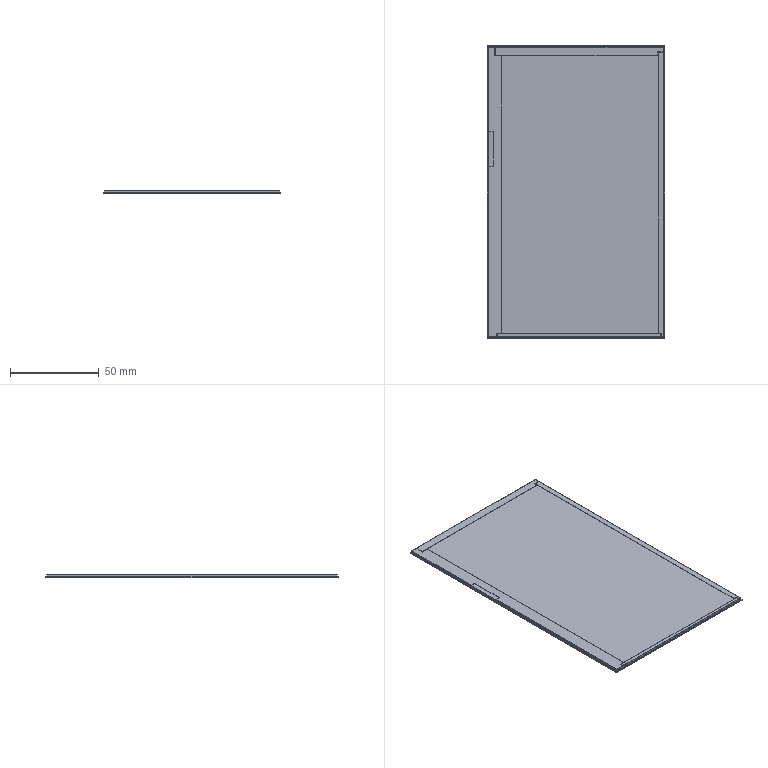Part | STEP file | DMG10600T070_01WTC_X2_8FEA658_1 | 1 solid | 48 faces | box 99.7 x 164.6 x 1.775 mm | volume 25129 mm3 | plane 48